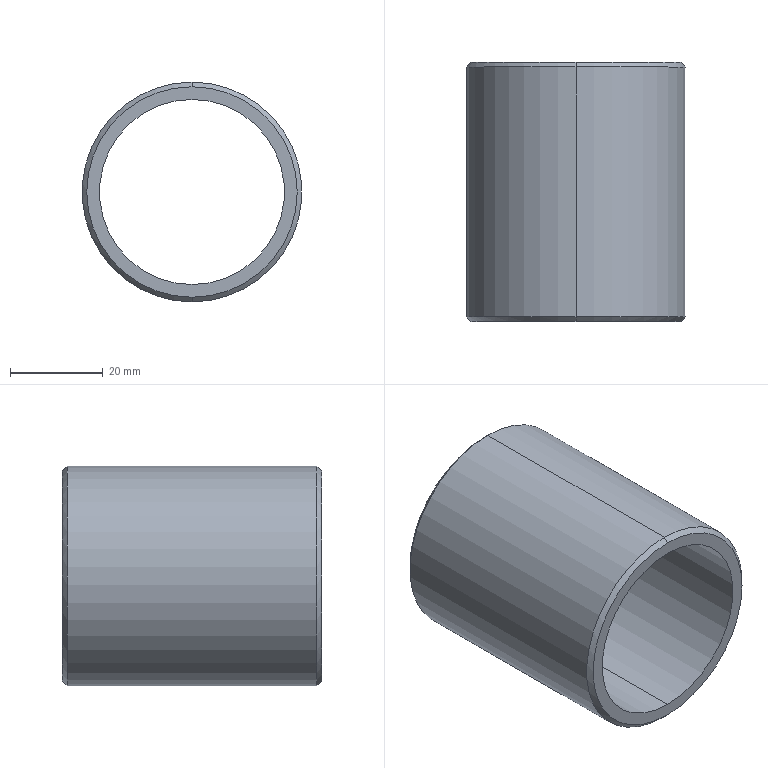Part | SolidWorks | features MBimport 1 | 1 solid | 10 faces | box 47.5 x 56 x 47.5 mm | volume 28716 mm3 | cone 4 | cylinder 4 | plane 2 | commonest cylinder face diameters 40 x2 47.5 x2
STEP:
#1=CARTESIAN_POINT('',(0.,-1.507,-22.75));
#2=VERTEX_POINT('',#1);
#3=CARTESIAN_POINT('',(0.,-0.5071,-23.75));
#4=VERTEX_POINT('',#3);
#5=CARTESIAN_POINT('',(0.,-1.507,-22.75));
#6=DIRECTION('',(0.,0.7071,-0.7071));
#7=VECTOR('',#6,1000.);
#8=LINE('',#5,#7);
#9=EDGE_CURVE('',#2,#4,#8,.T.);
#10=ORIENTED_EDGE('',*,*,#9,.F.);
#11=CARTESIAN_POINT('',(0.,-1.507,22.75));
#12=VERTEX_POINT('',#11);
#13=CARTESIAN_POINT('',(0.,-1.507,0.));
#14=DIRECTION('',(0.,-1.,0.));
#15=DIRECTION('',(0.,0.,1.));
#16=AXIS2_PLACEMENT_3D('',#13,#14,#15);
#17=CIRCLE('',#16,22.75);
#18=EDGE_CURVE('',#12,#2,#17,.T.);
#19=ORIENTED_EDGE('',*,*,#18,.F.);
#20=CARTESIAN_POINT('',(0.,-0.5071,23.75));
#21=VERTEX_POINT('',#20);
#22=CARTESIAN_POINT('',(0.,-1.507,22.75));
#23=DIRECTION('',(0.,0.7071,0.7071));
#24=VECTOR('',#23,1000.);
#25=LINE('',#22,#24);
#26=EDGE_CURVE('',#12,#21,#25,.T.);
#27=ORIENTED_EDGE('',*,*,#26,.T.);
#28=CARTESIAN_POINT('',(0.,-0.5071,0.));
#29=DIRECTION('',(0.,1.,0.));
#30=DIRECTION('',(0.,0.,1.));
#31=AXIS2_PLACEMENT_3D('',#28,#29,#30);
#32=CIRCLE('',#31,23.75);
#33=EDGE_CURVE('',#4,#21,#32,.T.);
#34=ORIENTED_EDGE('',*,*,#33,.F.);
#35=EDGE_LOOP('',(#10,#19,#27,#34));
#36=FACE_OUTER_BOUND('',#35,.T.);
#37=CARTESIAN_POINT('',(0.,-1.507,0.));
#38=DIRECTION('',(0.,1.,0.));
#39=DIRECTION('',(0.,0.,1.));
#40=AXIS2_PLACEMENT_3D('',#37,#38,#39);
#41=CONICAL_SURFACE('',#40,22.75,0.7854);
#42=ADVANCED_FACE('',(#36),#41,.T.);
#43=CARTESIAN_POINT('',(0.,54.493,22.75));
#44=VERTEX_POINT('',#43);
#45=CARTESIAN_POINT('',(0.,53.493,23.75));
#46=VERTEX_POINT('',#45);
#47=CARTESIAN_POINT('',(0.,53.493,23.75));
#48=DIRECTION('',(0.,-0.7071,0.7071));
#49=VECTOR('',#48,1000.);
#50=LINE('',#47,#49);
#51=EDGE_CURVE('',#44,#46,#50,.T.);
#52=ORIENTED_EDGE('',*,*,#51,.F.);
#53=CARTESIAN_POINT('',(0.,54.493,-22.75));
#54=VERTEX_POINT('',#53);
#55=CARTESIAN_POINT('',(0.,54.493,0.));
#56=DIRECTION('',(0.,1.,0.));
#57=DIRECTION('',(0.,0.,-1.));
#58=AXIS2_PLACEMENT_3D('',#55,#56,#57);
#59=CIRCLE('',#58,22.75);
#60=EDGE_CURVE('',#54,#44,#59,.T.);
#61=ORIENTED_EDGE('',*,*,#60,.F.);
#62=CARTESIAN_POINT('',(0.,53.493,-23.75));
#63=VERTEX_POINT('',#62);
#64=CARTESIAN_POINT('',(0.,53.493,-23.75));
#65=DIRECTION('',(0.,-0.7071,-0.7071));
#66=VECTOR('',#65,1000.);
#67=LINE('',#64,#66);
#68=EDGE_CURVE('',#54,#63,#67,.T.);
#69=ORIENTED_EDGE('',*,*,#68,.T.);
#70=CARTESIAN_POINT('',(0.,53.493,0.));
#71=DIRECTION('',(0.,-1.,0.));
#72=DIRECTION('',(0.,0.,-1.));
#73=AXIS2_PLACEMENT_3D('',#70,#71,#72);
#74=CIRCLE('',#73,23.75);
#75=EDGE_CURVE('',#46,#63,#74,.T.);
#76=ORIENTED_EDGE('',*,*,#75,.F.);
#77=EDGE_LOOP('',(#52,#61,#69,#76));
#78=FACE_OUTER_BOUND('',#77,.T.);
#79=CARTESIAN_POINT('',(0.,53.493,0.));
#80=DIRECTION('',(0.,-1.,0.));
#81=DIRECTION('',(0.,0.,-1.));
#82=AXIS2_PLACEMENT_3D('',#79,#80,#81);
#83=CONICAL_SURFACE('',#82,23.75,0.7854);
#84=ADVANCED_FACE('',(#78),#83,.T.);
#85=CARTESIAN_POINT('',(0.,54.493,-20.));
#86=VERTEX_POINT('',#85);
#87=CARTESIAN_POINT('',(0.,54.493,20.));
#88=VERTEX_POINT('',#87);
#89=CARTESIAN_POINT('',(0.,54.493,0.));
#90=DIRECTION('',(0.,-1.,0.));
#91=DIRECTION('',(0.,0.,-1.));
#92=AXIS2_PLACEMENT_3D('',#89,#90,#91);
#93=CIRCLE('',#92,20.);
#94=EDGE_CURVE('',#86,#88,#93,.T.);
#95=ORIENTED_EDGE('',*,*,#94,.T.);
#96=CARTESIAN_POINT('',(0.,54.493,0.));
#97=DIRECTION('',(0.,-1.,0.));
#98=DIRECTION('',(0.,0.,-1.));
#99=AXIS2_PLACEMENT_3D('',#96,#97,#98);
#100=CIRCLE('',#99,20.);
#101=EDGE_CURVE('',#88,#86,#100,.T.);
#102=ORIENTED_EDGE('',*,*,#101,.T.);
#103=EDGE_LOOP('',(#95,#102));
#104=FACE_BOUND('',#103,.T.);
#105=ORIENTED_EDGE('',*,*,#60,.T.);
#106=CARTESIAN_POINT('',(0.,54.493,0.));
#107=DIRECTION('',(0.,1.,0.));
#108=DIRECTION('',(0.,0.,-1.));
#109=AXIS2_PLACEMENT_3D('',#106,#107,#108);
#110=CIRCLE('',#109,22.75);
#111=EDGE_CURVE('',#44,#54,#110,.T.);
#112=ORIENTED_EDGE('',*,*,#111,.T.);
#113=EDGE_LOOP('',(#105,#112));
#114=FACE_OUTER_BOUND('',#113,.T.);
#115=CARTESIAN_POINT('',(-23.75,54.493,0.));
#116=DIRECTION('',(0.,-1.,0.));
#117=DIRECTION('',(0.,0.,-1.));
#118=AXIS2_PLACEMENT_3D('',#115,#116,#117);
#119=PLANE('',#118);
#120=ADVANCED_FACE('',(#104,#114),#119,.F.);
#121=CARTESIAN_POINT('',(0.,-1.507,20.));
#122=VERTEX_POINT('',#121);
#123=CARTESIAN_POINT('',(0.,0.,20.));
#124=DIRECTION('',(0.,-1.,0.));
#125=VECTOR('',#124,1000.);
#126=LINE('',#123,#125);
#127=EDGE_CURVE('',#88,#122,#126,.T.);
#128=ORIENTED_EDGE('',*,*,#127,.F.);
#129=ORIENTED_EDGE('',*,*,#94,.F.);
#130=CARTESIAN_POINT('',(0.,-1.507,-20.));
#131=VERTEX_POINT('',#130);
#132=CARTESIAN_POINT('',(0.,0.,-20.));
#133=DIRECTION('',(0.,-1.,0.));
#134=VECTOR('',#133,1000.);
#135=LINE('',#132,#134);
#136=EDGE_CURVE('',#86,#131,#135,.T.);
#137=ORIENTED_EDGE('',*,*,#136,.T.);
#138=CARTESIAN_POINT('',(0.,-1.507,0.));
#139=DIRECTION('',(0.,-1.,0.));
#140=DIRECTION('',(0.,0.,-1.));
#141=AXIS2_PLACEMENT_3D('',#138,#139,#140);
#142=CIRCLE('',#141,20.);
#143=EDGE_CURVE('',#131,#122,#142,.T.);
#144=ORIENTED_EDGE('',*,*,#143,.T.);
#145=EDGE_LOOP('',(#128,#129,#137,#144));
#146=FACE_OUTER_BOUND('',#145,.T.);
#147=CARTESIAN_POINT('',(0.,0.,0.));
#148=DIRECTION('',(0.,-1.,0.));
#149=DIRECTION('',(0.,0.,-1.));
#150=AXIS2_PLACEMENT_3D('',#147,#148,#149);
#151=CYLINDRICAL_SURFACE('',#150,20.);
#152=ADVANCED_FACE('',(#146),#151,.F.);
#153=ORIENTED_EDGE('',*,*,#143,.F.);
#154=CARTESIAN_POINT('',(0.,-1.507,0.));
#155=DIRECTION('',(0.,-1.,0.));
#156=DIRECTION('',(0.,0.,-1.));
#157=AXIS2_PLACEMENT_3D('',#154,#155,#156);
#158=CIRCLE('',#157,20.);
#159=EDGE_CURVE('',#122,#131,#158,.T.);
#160=ORIENTED_EDGE('',*,*,#159,.F.);
#161=EDGE_LOOP('',(#153,#160));
#162=FACE_BOUND('',#161,.T.);
#163=ORIENTED_EDGE('',*,*,#18,.T.);
#164=CARTESIAN_POINT('',(0.,-1.507,0.));
#165=DIRECTION('',(0.,-1.,0.));
#166=DIRECTION('',(0.,0.,1.));
#167=AXIS2_PLACEMENT_3D('',#164,#165,#166);
#168=CIRCLE('',#167,22.75);
#169=EDGE_CURVE('',#2,#12,#168,.T.);
#170=ORIENTED_EDGE('',*,*,#169,.T.);
#171=EDGE_LOOP('',(#163,#170));
#172=FACE_OUTER_BOUND('',#171,.T.);
#173=CARTESIAN_POINT('',(-23.75,-1.507,0.));
#174=DIRECTION('',(0.,1.,0.));
#175=DIRECTION('',(1.,0.,0.));
#176=AXIS2_PLACEMENT_3D('',#173,#174,#175);
#177=PLANE('',#176);
#178=ADVANCED_FACE('',(#162,#172),#177,.F.);
#179=CARTESIAN_POINT('',(0.,0.,23.75));
#180=DIRECTION('',(0.,-1.,0.));
#181=VECTOR('',#180,1000.);
#182=LINE('',#179,#181);
#183=EDGE_CURVE('',#46,#21,#182,.T.);
#184=ORIENTED_EDGE('',*,*,#183,.F.);
#185=ORIENTED_EDGE('',*,*,#75,.T.);
#186=CARTESIAN_POINT('',(0.,0.,-23.75));
#187=DIRECTION('',(0.,-1.,0.));
#188=VECTOR('',#187,1000.);
#189=LINE('',#186,#188);
#190=EDGE_CURVE('',#63,#4,#189,.T.);
#191=ORIENTED_EDGE('',*,*,#190,.T.);
#192=ORIENTED_EDGE('',*,*,#33,.T.);
#193=EDGE_LOOP('',(#184,#185,#191,#192));
#194=FACE_OUTER_BOUND('',#193,.T.);
#195=CARTESIAN_POINT('',(0.,0.,0.));
#196=DIRECTION('',(0.,-1.,0.));
#197=DIRECTION('',(0.,0.,-1.));
#198=AXIS2_PLACEMENT_3D('',#195,#196,#197);
#199=CYLINDRICAL_SURFACE('',#198,23.75);
#200=ADVANCED_FACE('',(#194),#199,.T.);
#201=CARTESIAN_POINT('',(0.,53.493,0.));
#202=DIRECTION('',(0.,-1.,0.));
#203=DIRECTION('',(0.,0.,-1.));
#204=AXIS2_PLACEMENT_3D('',#201,#202,#203);
#205=CIRCLE('',#204,23.75);
#206=EDGE_CURVE('',#63,#46,#205,.T.);
#207=ORIENTED_EDGE('',*,*,#206,.T.);
#208=ORIENTED_EDGE('',*,*,#183,.T.);
#209=CARTESIAN_POINT('',(0.,-0.5071,0.));
#210=DIRECTION('',(0.,1.,0.));
#211=DIRECTION('',(0.,0.,1.));
#212=AXIS2_PLACEMENT_3D('',#209,#210,#211);
#213=CIRCLE('',#212,23.75);
#214=EDGE_CURVE('',#21,#4,#213,.T.);
#215=ORIENTED_EDGE('',*,*,#214,.T.);
#216=ORIENTED_EDGE('',*,*,#190,.F.);
#217=EDGE_LOOP('',(#207,#208,#215,#216));
#218=FACE_OUTER_BOUND('',#217,.T.);
#219=CARTESIAN_POINT('',(0.,0.,0.));
#220=DIRECTION('',(0.,-1.,0.));
#221=DIRECTION('',(0.,0.,-1.));
#222=AXIS2_PLACEMENT_3D('',#219,#220,#221);
#223=CYLINDRICAL_SURFACE('',#222,23.75);
#224=ADVANCED_FACE('',(#218),#223,.T.);
#225=ORIENTED_EDGE('',*,*,#101,.F.);
#226=ORIENTED_EDGE('',*,*,#127,.T.);
#227=ORIENTED_EDGE('',*,*,#159,.T.);
#228=ORIENTED_EDGE('',*,*,#136,.F.);
#229=EDGE_LOOP('',(#225,#226,#227,#228));
#230=FACE_OUTER_BOUND('',#229,.T.);
#231=CARTESIAN_POINT('',(0.,0.,0.));
#232=DIRECTION('',(0.,-1.,0.));
#233=DIRECTION('',(0.,0.,-1.));
#234=AXIS2_PLACEMENT_3D('',#231,#232,#233);
#235=CYLINDRICAL_SURFACE('',#234,20.);
#236=ADVANCED_FACE('',(#230),#235,.F.);
#237=ORIENTED_EDGE('',*,*,#111,.F.);
#238=ORIENTED_EDGE('',*,*,#51,.T.);
#239=ORIENTED_EDGE('',*,*,#206,.F.);
#240=ORIENTED_EDGE('',*,*,#68,.F.);
#241=EDGE_LOOP('',(#237,#238,#239,#240));
#242=FACE_OUTER_BOUND('',#241,.T.);
#243=CARTESIAN_POINT('',(0.,53.493,0.));
#244=DIRECTION('',(0.,-1.,0.));
#245=DIRECTION('',(0.,0.,-1.));
#246=AXIS2_PLACEMENT_3D('',#243,#244,#245);
#247=CONICAL_SURFACE('',#246,23.75,0.7854);
#248=ADVANCED_FACE('',(#242),#247,.T.);
#249=ORIENTED_EDGE('',*,*,#169,.F.);
#250=ORIENTED_EDGE('',*,*,#9,.T.);
#251=ORIENTED_EDGE('',*,*,#214,.F.);
#252=ORIENTED_EDGE('',*,*,#26,.F.);
#253=EDGE_LOOP('',(#249,#250,#251,#252));
#254=FACE_OUTER_BOUND('',#253,.T.);
#255=CARTESIAN_POINT('',(0.,-1.507,0.));
#256=DIRECTION('',(0.,1.,0.));
#257=DIRECTION('',(0.,0.,1.));
#258=AXIS2_PLACEMENT_3D('',#255,#256,#257);
#259=CONICAL_SURFACE('',#258,22.75,0.7854);
#260=ADVANCED_FACE('',(#254),#259,.T.);
#261=CLOSED_SHELL('',(#42,#84,#120,#152,#178,#200,#224,#236,#248,#260));
#262=MANIFOLD_SOLID_BREP('',#261);
#263=CARTESIAN_POINT('',(0.,0.,0.));
#264=DIRECTION('',(0.,0.,1.));
#265=DIRECTION('',(1.,0.,0.));
#266=AXIS2_PLACEMENT_3D('',#263,#264,#265);
#267=(LENGTH_UNIT()NAMED_UNIT(*)SI_UNIT(.MILLI.,.METRE.));
#268=UNCERTAINTY_MEASURE_WITH_UNIT(LENGTH_MEASURE(0.00001),#267,'','');
#269=(NAMED_UNIT(*)PLANE_ANGLE_UNIT()SI_UNIT($,.RADIAN.));
#270=(NAMED_UNIT(*)SI_UNIT($,.STERADIAN.)SOLID_ANGLE_UNIT());
#271=(GEOMETRIC_REPRESENTATION_CONTEXT(3)GLOBAL_UNCERTAINTY_ASSIGNED_CONTEXT((#268))GLOBAL_UNIT_ASSIGNED_CONTEXT((#267,#269,#270))REPRESENTATION_CONTEXT('',''));
#272=ADVANCED_BREP_SHAPE_REPRESENTATION('',(#262,#266),#271);